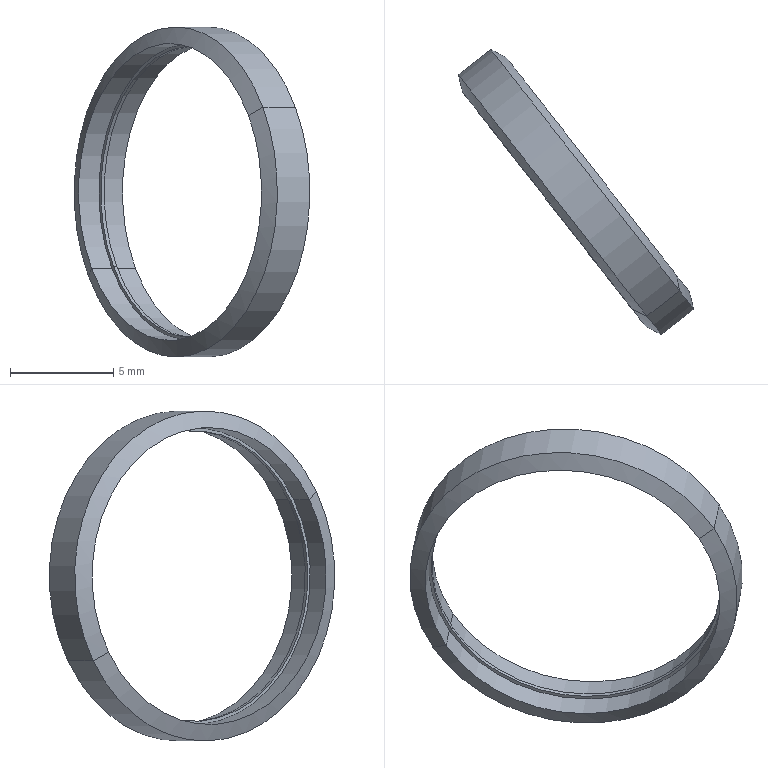Part | SolidWorks | features BaseBody 1 | 1 solid | 14 faces | box 11.427 x 13.839 x 16 mm | volume 90.883 mm3 | cylinder 8 | cone 4 | plane 2 | commonest cylinder face diameters 14.4 x4 14.1 x2 16 x2
STEP:
#1=CARTESIAN_POINT('',(7.125,91.055,73.948));
#2=VERTEX_POINT('',#1);
#3=CARTESIAN_POINT('',(-0.4819,100.792,66.552));
#4=VERTEX_POINT('',#3);
#5=CARTESIAN_POINT('',(3.322,95.923,70.25));
#6=DIRECTION('',(0.788,0.6157,0.));
#7=DIRECTION('',(-0.5283,0.6761,-0.5136));
#8=AXIS2_PLACEMENT_3D('',#5,#6,#7);
#9=CIRCLE('',#8,7.2);
#10=EDGE_CURVE('',#2,#4,#9,.T.);
#11=ORIENTED_EDGE('',*,*,#10,.F.);
#12=CARTESIAN_POINT('',(8.11,91.825,73.948));
#13=VERTEX_POINT('',#12);
#14=CARTESIAN_POINT('',(17.851,99.435,73.948));
#15=DIRECTION('',(0.788,0.6157,0.));
#16=VECTOR('',#15,1000.);
#17=LINE('',#14,#16);
#18=EDGE_CURVE('',#2,#13,#17,.T.);
#19=ORIENTED_EDGE('',*,*,#18,.T.);
#20=CARTESIAN_POINT('',(0.5031,101.561,66.552));
#21=VERTEX_POINT('',#20);
#22=CARTESIAN_POINT('',(4.307,96.693,70.25));
#23=DIRECTION('',(0.788,0.6157,0.));
#24=DIRECTION('',(-0.5283,0.6761,-0.5136));
#25=AXIS2_PLACEMENT_3D('',#22,#23,#24);
#26=CIRCLE('',#25,7.2);
#27=EDGE_CURVE('',#13,#21,#26,.T.);
#28=ORIENTED_EDGE('',*,*,#27,.T.);
#29=CARTESIAN_POINT('',(10.244,109.171,66.552));
#30=DIRECTION('',(0.788,0.6157,0.));
#31=VECTOR('',#30,1000.);
#32=LINE('',#29,#31);
#33=EDGE_CURVE('',#4,#21,#32,.T.);
#34=ORIENTED_EDGE('',*,*,#33,.F.);
#35=EDGE_LOOP('',(#11,#19,#28,#34));
#36=FACE_OUTER_BOUND('',#35,.T.);
#37=CARTESIAN_POINT('',(14.047,104.303,70.25));
#38=DIRECTION('',(0.788,0.6157,0.));
#39=DIRECTION('',(-0.5283,0.6761,-0.5136));
#40=AXIS2_PLACEMENT_3D('',#37,#38,#39);
#41=CYLINDRICAL_SURFACE('',#40,7.2);
#42=ADVANCED_FACE('',(#36),#41,.F.);
#43=CARTESIAN_POINT('',(3.322,95.923,70.25));
#44=DIRECTION('',(0.788,0.6157,0.));
#45=DIRECTION('',(-0.5283,0.6761,-0.5136));
#46=AXIS2_PLACEMENT_3D('',#43,#44,#45);
#47=CIRCLE('',#46,7.2);
#48=EDGE_CURVE('',#4,#2,#47,.T.);
#49=ORIENTED_EDGE('',*,*,#48,.T.);
#50=CARTESIAN_POINT('',(7.823,90.73,74.359));
#51=VERTEX_POINT('',#50);
#52=CARTESIAN_POINT('',(7.125,91.055,73.948));
#53=DIRECTION('',(0.7998,-0.3727,0.4705));
#54=VECTOR('',#53,1000.);
#55=LINE('',#52,#54);
#56=EDGE_CURVE('',#2,#51,#55,.T.);
#57=ORIENTED_EDGE('',*,*,#56,.T.);
#58=CARTESIAN_POINT('',(-0.6287,101.548,66.141));
#59=VERTEX_POINT('',#58);
#60=CARTESIAN_POINT('',(3.597,96.139,70.25));
#61=DIRECTION('',(0.788,0.6157,0.));
#62=DIRECTION('',(-0.5283,0.6761,-0.5136));
#63=AXIS2_PLACEMENT_3D('',#60,#61,#62);
#64=CIRCLE('',#63,8.);
#65=EDGE_CURVE('',#59,#51,#64,.T.);
#66=ORIENTED_EDGE('',*,*,#65,.F.);
#67=CARTESIAN_POINT('',(-0.4819,100.792,66.552));
#68=DIRECTION('',(-0.1681,0.8662,-0.4705));
#69=VECTOR('',#68,1000.);
#70=LINE('',#67,#69);
#71=EDGE_CURVE('',#4,#59,#70,.T.);
#72=ORIENTED_EDGE('',*,*,#71,.F.);
#73=EDGE_LOOP('',(#49,#57,#66,#72));
#74=FACE_OUTER_BOUND('',#73,.T.);
#75=CARTESIAN_POINT('',(3.322,95.923,70.25));
#76=DIRECTION('',(0.788,0.6157,0.));
#77=DIRECTION('',(-0.5283,0.6761,-0.5136));
#78=AXIS2_PLACEMENT_3D('',#75,#76,#77);
#79=CONICAL_SURFACE('',#78,7.2,1.158);
#80=ADVANCED_FACE('',(#74),#79,.T.);
#81=ORIENTED_EDGE('',*,*,#65,.T.);
#82=CARTESIAN_POINT('',(9.399,91.961,74.359));
#83=VERTEX_POINT('',#82);
#84=CARTESIAN_POINT('',(18.273,98.894,74.359));
#85=DIRECTION('',(0.788,0.6157,0.));
#86=VECTOR('',#85,1000.);
#87=LINE('',#84,#86);
#88=EDGE_CURVE('',#51,#83,#87,.T.);
#89=ORIENTED_EDGE('',*,*,#88,.T.);
#90=CARTESIAN_POINT('',(0.9473,102.779,66.141));
#91=VERTEX_POINT('',#90);
#92=CARTESIAN_POINT('',(5.173,97.37,70.25));
#93=DIRECTION('',(0.788,0.6157,0.));
#94=DIRECTION('',(-0.5283,0.6761,-0.5136));
#95=AXIS2_PLACEMENT_3D('',#92,#93,#94);
#96=CIRCLE('',#95,8.);
#97=EDGE_CURVE('',#91,#83,#96,.T.);
#98=ORIENTED_EDGE('',*,*,#97,.F.);
#99=CARTESIAN_POINT('',(9.821,109.712,66.141));
#100=DIRECTION('',(0.788,0.6157,0.));
#101=VECTOR('',#100,1000.);
#102=LINE('',#99,#101);
#103=EDGE_CURVE('',#59,#91,#102,.T.);
#104=ORIENTED_EDGE('',*,*,#103,.F.);
#105=EDGE_LOOP('',(#81,#89,#98,#104));
#106=FACE_OUTER_BOUND('',#105,.T.);
#107=CARTESIAN_POINT('',(14.047,104.303,70.25));
#108=DIRECTION('',(0.788,0.6157,0.));
#109=DIRECTION('',(-0.5283,0.6761,-0.5136));
#110=AXIS2_PLACEMENT_3D('',#107,#108,#109);
#111=CYLINDRICAL_SURFACE('',#110,8.);
#112=ADVANCED_FACE('',(#106),#111,.T.);
#113=CARTESIAN_POINT('',(1.646,102.454,66.552));
#114=VERTEX_POINT('',#113);
#115=CARTESIAN_POINT('',(9.253,92.718,73.948));
#116=VERTEX_POINT('',#115);
#117=CARTESIAN_POINT('',(5.449,97.586,70.25));
#118=DIRECTION('',(0.788,0.6157,0.));
#119=DIRECTION('',(-0.5283,0.6761,-0.5136));
#120=AXIS2_PLACEMENT_3D('',#117,#118,#119);
#121=CIRCLE('',#120,7.2);
#122=EDGE_CURVE('',#114,#116,#121,.T.);
#123=ORIENTED_EDGE('',*,*,#122,.F.);
#124=CARTESIAN_POINT('',(0.9473,102.779,66.141));
#125=DIRECTION('',(-0.7998,0.3727,-0.4705));
#126=VECTOR('',#125,1000.);
#127=LINE('',#124,#126);
#128=EDGE_CURVE('',#114,#91,#127,.T.);
#129=ORIENTED_EDGE('',*,*,#128,.T.);
#130=ORIENTED_EDGE('',*,*,#97,.T.);
#131=CARTESIAN_POINT('',(9.399,91.961,74.359));
#132=DIRECTION('',(0.1681,-0.8662,0.4705));
#133=VECTOR('',#132,1000.);
#134=LINE('',#131,#133);
#135=EDGE_CURVE('',#116,#83,#134,.T.);
#136=ORIENTED_EDGE('',*,*,#135,.F.);
#137=EDGE_LOOP('',(#123,#129,#130,#136));
#138=FACE_OUTER_BOUND('',#137,.T.);
#139=CARTESIAN_POINT('',(5.173,97.37,70.25));
#140=DIRECTION('',(-0.788,-0.6157,0.));
#141=DIRECTION('',(0.5283,-0.6761,0.5136));
#142=AXIS2_PLACEMENT_3D('',#139,#140,#141);
#143=CONICAL_SURFACE('',#142,8.,1.158);
#144=ADVANCED_FACE('',(#138),#143,.T.);
#145=CARTESIAN_POINT('',(8.268,91.948,73.948));
#146=VERTEX_POINT('',#145);
#147=CARTESIAN_POINT('',(0.6607,101.684,66.552));
#148=VERTEX_POINT('',#147);
#149=CARTESIAN_POINT('',(4.464,96.816,70.25));
#150=DIRECTION('',(0.788,0.6157,0.));
#151=DIRECTION('',(-0.5283,0.6761,-0.5136));
#152=AXIS2_PLACEMENT_3D('',#149,#150,#151);
#153=CIRCLE('',#152,7.2);
#154=EDGE_CURVE('',#146,#148,#153,.T.);
#155=ORIENTED_EDGE('',*,*,#154,.F.);
#156=CARTESIAN_POINT('',(17.851,99.435,73.948));
#157=DIRECTION('',(0.788,0.6157,0.));
#158=VECTOR('',#157,1000.);
#159=LINE('',#156,#158);
#160=EDGE_CURVE('',#146,#116,#159,.T.);
#161=ORIENTED_EDGE('',*,*,#160,.T.);
#162=CARTESIAN_POINT('',(5.449,97.586,70.25));
#163=DIRECTION('',(0.788,0.6157,0.));
#164=DIRECTION('',(-0.5283,0.6761,-0.5136));
#165=AXIS2_PLACEMENT_3D('',#162,#163,#164);
#166=CIRCLE('',#165,7.2);
#167=EDGE_CURVE('',#116,#114,#166,.T.);
#168=ORIENTED_EDGE('',*,*,#167,.T.);
#169=CARTESIAN_POINT('',(10.244,109.171,66.552));
#170=DIRECTION('',(0.788,0.6157,0.));
#171=VECTOR('',#170,1000.);
#172=LINE('',#169,#171);
#173=EDGE_CURVE('',#148,#114,#172,.T.);
#174=ORIENTED_EDGE('',*,*,#173,.F.);
#175=EDGE_LOOP('',(#155,#161,#168,#174));
#176=FACE_OUTER_BOUND('',#175,.T.);
#177=CARTESIAN_POINT('',(14.047,104.303,70.25));
#178=DIRECTION('',(0.788,0.6157,0.));
#179=DIRECTION('',(-0.5283,0.6761,-0.5136));
#180=AXIS2_PLACEMENT_3D('',#177,#178,#179);
#181=CYLINDRICAL_SURFACE('',#180,7.2);
#182=ADVANCED_FACE('',(#176),#181,.F.);
#183=CARTESIAN_POINT('',(8.031,91.926,73.871));
#184=VERTEX_POINT('',#183);
#185=CARTESIAN_POINT('',(0.5824,101.46,66.629));
#186=VERTEX_POINT('',#185);
#187=CARTESIAN_POINT('',(4.307,96.693,70.25));
#188=DIRECTION('',(0.788,0.6157,0.));
#189=DIRECTION('',(-0.5283,0.6761,-0.5136));
#190=AXIS2_PLACEMENT_3D('',#187,#188,#189);
#191=CIRCLE('',#190,7.05);
#192=EDGE_CURVE('',#184,#186,#191,.T.);
#193=ORIENTED_EDGE('',*,*,#192,.F.);
#194=CARTESIAN_POINT('',(8.188,92.049,73.871));
#195=VERTEX_POINT('',#194);
#196=CARTESIAN_POINT('',(17.771,99.536,73.871));
#197=DIRECTION('',(0.788,0.6157,0.));
#198=VECTOR('',#197,1000.);
#199=LINE('',#196,#198);
#200=EDGE_CURVE('',#184,#195,#199,.T.);
#201=ORIENTED_EDGE('',*,*,#200,.T.);
#202=CARTESIAN_POINT('',(0.74,101.583,66.629));
#203=VERTEX_POINT('',#202);
#204=CARTESIAN_POINT('',(4.464,96.816,70.25));
#205=DIRECTION('',(0.788,0.6157,0.));
#206=DIRECTION('',(-0.5283,0.6761,-0.5136));
#207=AXIS2_PLACEMENT_3D('',#204,#205,#206);
#208=CIRCLE('',#207,7.05);
#209=EDGE_CURVE('',#195,#203,#208,.T.);
#210=ORIENTED_EDGE('',*,*,#209,.T.);
#211=CARTESIAN_POINT('',(10.323,109.07,66.629));
#212=DIRECTION('',(0.788,0.6157,0.));
#213=VECTOR('',#212,1000.);
#214=LINE('',#211,#213);
#215=EDGE_CURVE('',#186,#203,#214,.T.);
#216=ORIENTED_EDGE('',*,*,#215,.F.);
#217=EDGE_LOOP('',(#193,#201,#210,#216));
#218=FACE_OUTER_BOUND('',#217,.T.);
#219=CARTESIAN_POINT('',(14.047,104.303,70.25));
#220=DIRECTION('',(0.788,0.6157,0.));
#221=DIRECTION('',(-0.5283,0.6761,-0.5136));
#222=AXIS2_PLACEMENT_3D('',#219,#220,#221);
#223=CYLINDRICAL_SURFACE('',#222,7.05);
#224=ADVANCED_FACE('',(#218),#223,.F.);
#225=CARTESIAN_POINT('',(4.307,96.693,70.25));
#226=DIRECTION('',(0.788,0.6157,0.));
#227=DIRECTION('',(-0.5283,0.6761,-0.5136));
#228=AXIS2_PLACEMENT_3D('',#225,#226,#227);
#229=CIRCLE('',#228,7.05);
#230=EDGE_CURVE('',#186,#184,#229,.T.);
#231=ORIENTED_EDGE('',*,*,#230,.T.);
#232=ORIENTED_EDGE('',*,*,#192,.T.);
#233=EDGE_LOOP('',(#231,#232));
#234=FACE_BOUND('',#233,.T.);
#235=CARTESIAN_POINT('',(4.307,96.693,70.25));
#236=DIRECTION('',(0.788,0.6157,0.));
#237=DIRECTION('',(-0.5283,0.6761,-0.5136));
#238=AXIS2_PLACEMENT_3D('',#235,#236,#237);
#239=CIRCLE('',#238,7.2);
#240=EDGE_CURVE('',#21,#13,#239,.T.);
#241=ORIENTED_EDGE('',*,*,#240,.F.);
#242=ORIENTED_EDGE('',*,*,#27,.F.);
#243=EDGE_LOOP('',(#241,#242));
#244=FACE_OUTER_BOUND('',#243,.T.);
#245=CARTESIAN_POINT('',(6.583,93.779,64.072));
#246=DIRECTION('',(0.788,0.6157,0.));
#247=DIRECTION('',(0.,0.,-1.));
#248=AXIS2_PLACEMENT_3D('',#245,#246,#247);
#249=PLANE('',#248);
#250=ADVANCED_FACE('',(#234,#244),#249,.F.);
#251=ORIENTED_EDGE('',*,*,#200,.F.);
#252=ORIENTED_EDGE('',*,*,#230,.F.);
#253=ORIENTED_EDGE('',*,*,#215,.T.);
#254=CARTESIAN_POINT('',(4.464,96.816,70.25));
#255=DIRECTION('',(0.788,0.6157,0.));
#256=DIRECTION('',(-0.5283,0.6761,-0.5136));
#257=AXIS2_PLACEMENT_3D('',#254,#255,#256);
#258=CIRCLE('',#257,7.05);
#259=EDGE_CURVE('',#203,#195,#258,.T.);
#260=ORIENTED_EDGE('',*,*,#259,.T.);
#261=EDGE_LOOP('',(#251,#252,#253,#260));
#262=FACE_OUTER_BOUND('',#261,.T.);
#263=CARTESIAN_POINT('',(14.047,104.303,70.25));
#264=DIRECTION('',(0.788,0.6157,0.));
#265=DIRECTION('',(-0.5283,0.6761,-0.5136));
#266=AXIS2_PLACEMENT_3D('',#263,#264,#265);
#267=CYLINDRICAL_SURFACE('',#266,7.05);
#268=ADVANCED_FACE('',(#262),#267,.F.);
#269=CARTESIAN_POINT('',(4.464,96.816,70.25));
#270=DIRECTION('',(0.788,0.6157,0.));
#271=DIRECTION('',(-0.5283,0.6761,-0.5136));
#272=AXIS2_PLACEMENT_3D('',#269,#270,#271);
#273=CIRCLE('',#272,7.2);
#274=EDGE_CURVE('',#148,#146,#273,.T.);
#275=ORIENTED_EDGE('',*,*,#274,.T.);
#276=ORIENTED_EDGE('',*,*,#154,.T.);
#277=EDGE_LOOP('',(#275,#276));
#278=FACE_OUTER_BOUND('',#277,.T.);
#279=ORIENTED_EDGE('',*,*,#259,.F.);
#280=ORIENTED_EDGE('',*,*,#209,.F.);
#281=EDGE_LOOP('',(#279,#280));
#282=FACE_BOUND('',#281,.T.);
#283=CARTESIAN_POINT('',(6.741,93.902,64.072));
#284=DIRECTION('',(-0.788,-0.6157,0.));
#285=DIRECTION('',(-0.6157,0.788,0.));
#286=AXIS2_PLACEMENT_3D('',#283,#284,#285);
#287=PLANE('',#286);
#288=ADVANCED_FACE('',(#278,#282),#287,.F.);
#289=ORIENTED_EDGE('',*,*,#160,.F.);
#290=ORIENTED_EDGE('',*,*,#274,.F.);
#291=ORIENTED_EDGE('',*,*,#173,.T.);
#292=ORIENTED_EDGE('',*,*,#122,.T.);
#293=EDGE_LOOP('',(#289,#290,#291,#292));
#294=FACE_OUTER_BOUND('',#293,.T.);
#295=CARTESIAN_POINT('',(14.047,104.303,70.25));
#296=DIRECTION('',(0.788,0.6157,0.));
#297=DIRECTION('',(-0.5283,0.6761,-0.5136));
#298=AXIS2_PLACEMENT_3D('',#295,#296,#297);
#299=CYLINDRICAL_SURFACE('',#298,7.2);
#300=ADVANCED_FACE('',(#294),#299,.F.);
#301=ORIENTED_EDGE('',*,*,#128,.F.);
#302=ORIENTED_EDGE('',*,*,#167,.F.);
#303=ORIENTED_EDGE('',*,*,#135,.T.);
#304=CARTESIAN_POINT('',(5.173,97.37,70.25));
#305=DIRECTION('',(0.788,0.6157,0.));
#306=DIRECTION('',(-0.5283,0.6761,-0.5136));
#307=AXIS2_PLACEMENT_3D('',#304,#305,#306);
#308=CIRCLE('',#307,8.);
#309=EDGE_CURVE('',#83,#91,#308,.T.);
#310=ORIENTED_EDGE('',*,*,#309,.T.);
#311=EDGE_LOOP('',(#301,#302,#303,#310));
#312=FACE_OUTER_BOUND('',#311,.T.);
#313=CARTESIAN_POINT('',(5.173,97.37,70.25));
#314=DIRECTION('',(-0.788,-0.6157,0.));
#315=DIRECTION('',(0.5283,-0.6761,0.5136));
#316=AXIS2_PLACEMENT_3D('',#313,#314,#315);
#317=CONICAL_SURFACE('',#316,8.,1.158);
#318=ADVANCED_FACE('',(#312),#317,.T.);
#319=ORIENTED_EDGE('',*,*,#88,.F.);
#320=CARTESIAN_POINT('',(3.597,96.139,70.25));
#321=DIRECTION('',(0.788,0.6157,0.));
#322=DIRECTION('',(-0.5283,0.6761,-0.5136));
#323=AXIS2_PLACEMENT_3D('',#320,#321,#322);
#324=CIRCLE('',#323,8.);
#325=EDGE_CURVE('',#51,#59,#324,.T.);
#326=ORIENTED_EDGE('',*,*,#325,.T.);
#327=ORIENTED_EDGE('',*,*,#103,.T.);
#328=ORIENTED_EDGE('',*,*,#309,.F.);
#329=EDGE_LOOP('',(#319,#326,#327,#328));
#330=FACE_OUTER_BOUND('',#329,.T.);
#331=CARTESIAN_POINT('',(14.047,104.303,70.25));
#332=DIRECTION('',(0.788,0.6157,0.));
#333=DIRECTION('',(-0.5283,0.6761,-0.5136));
#334=AXIS2_PLACEMENT_3D('',#331,#332,#333);
#335=CYLINDRICAL_SURFACE('',#334,8.);
#336=ADVANCED_FACE('',(#330),#335,.T.);
#337=ORIENTED_EDGE('',*,*,#56,.F.);
#338=ORIENTED_EDGE('',*,*,#10,.T.);
#339=ORIENTED_EDGE('',*,*,#71,.T.);
#340=ORIENTED_EDGE('',*,*,#325,.F.);
#341=EDGE_LOOP('',(#337,#338,#339,#340));
#342=FACE_OUTER_BOUND('',#341,.T.);
#343=CARTESIAN_POINT('',(3.322,95.923,70.25));
#344=DIRECTION('',(0.788,0.6157,0.));
#345=DIRECTION('',(-0.5283,0.6761,-0.5136));
#346=AXIS2_PLACEMENT_3D('',#343,#344,#345);
#347=CONICAL_SURFACE('',#346,7.2,1.158);
#348=ADVANCED_FACE('',(#342),#347,.T.);
#349=ORIENTED_EDGE('',*,*,#18,.F.);
#350=ORIENTED_EDGE('',*,*,#48,.F.);
#351=ORIENTED_EDGE('',*,*,#33,.T.);
#352=ORIENTED_EDGE('',*,*,#240,.T.);
#353=EDGE_LOOP('',(#349,#350,#351,#352));
#354=FACE_OUTER_BOUND('',#353,.T.);
#355=CARTESIAN_POINT('',(14.047,104.303,70.25));
#356=DIRECTION('',(0.788,0.6157,0.));
#357=DIRECTION('',(-0.5283,0.6761,-0.5136));
#358=AXIS2_PLACEMENT_3D('',#355,#356,#357);
#359=CYLINDRICAL_SURFACE('',#358,7.2);
#360=ADVANCED_FACE('',(#354),#359,.F.);
#361=CLOSED_SHELL('',(#42,#80,#112,#144,#182,#224,#250,#268,#288,#300,#318,#336,#348,#360));
#362=MANIFOLD_SOLID_BREP('',#361);
#363=CARTESIAN_POINT('',(0.,0.,0.));
#364=DIRECTION('',(0.,0.,1.));
#365=DIRECTION('',(1.,0.,0.));
#366=AXIS2_PLACEMENT_3D('',#363,#364,#365);
#367=(LENGTH_UNIT()NAMED_UNIT(*)SI_UNIT(.MILLI.,.METRE.));
#368=UNCERTAINTY_MEASURE_WITH_UNIT(LENGTH_MEASURE(0.00001),#367,'','');
#369=(NAMED_UNIT(*)PLANE_ANGLE_UNIT()SI_UNIT($,.RADIAN.));
#370=(NAMED_UNIT(*)SI_UNIT($,.STERADIAN.)SOLID_ANGLE_UNIT());
#371=(GEOMETRIC_REPRESENTATION_CONTEXT(3)GLOBAL_UNCERTAINTY_ASSIGNED_CONTEXT((#368))GLOBAL_UNIT_ASSIGNED_CONTEXT((#367,#369,#370))REPRESENTATION_CONTEXT('',''));
#372=ADVANCED_BREP_SHAPE_REPRESENTATION('',(#362,#366),#371);